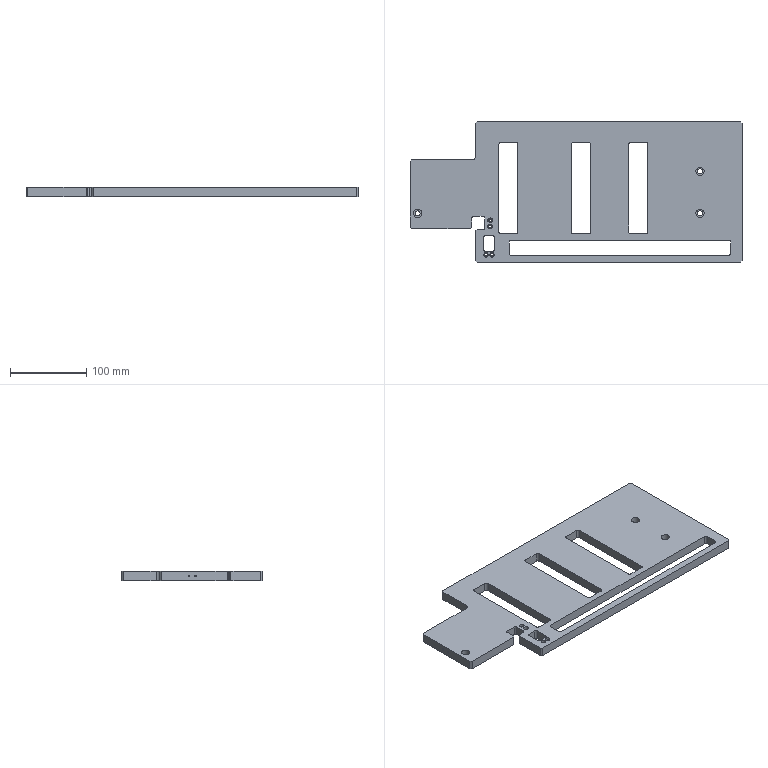NC program | NX | posted with a generic post | part box 435 x 184 x 12 mm
Lines 6316 to 7223 of 10210:
(HOLE_MILLING_COPY , TOOL : D4)
N12564 T11 M6
N12566 G54
N12568 G17 G0 G90 X-112.5 Y-37. S9500 M3
N12570 G43 Z30. H11
N12572 Z1.
N12574 G94 G3 X-112. Y-37.5 R0.5 F1500.
N12576 X-111.5 Y-37. R0.5
N12578 X-111.5 Y-37. Z0.5 I-1. J0.
N12580 X-111.5 Y-37. Z0. I-1. J0.
N12582 X-111.5 Y-37. Z-0.5 I-1. J0.
N12584 X-111.5 Y-37. Z-1. I-1. J0.
N12586 X-111.5 Y-37. Z-1.5 I-1. J0.
N12588 X-111.5 Y-37. Z-2. I-1. J0.
N12590 X-111.5 Y-37. Z-2.5 I-1. J0.
N12592 X-111.5 Y-37. Z-3. I-1. J0.
N12594 X-111.5 Y-37. Z-3.5 I-1. J0.
N12596 X-112.5 Y-36. R1.
N12598 X-111.5 Y-37. R-1.
N12600 X-112. Y-36.5 R0.5
N12602 X-112.5 Y-37. R0.5
N12604 G0 Z30.
N12606 Y-45.
N12608 Z1.
N12610 G3 X-112. Y-45.5 R0.5
N12612 X-111.5 Y-45. R0.5
N12614 X-111.5 Y-45. Z0.5 I-1. J0.
N12616 X-111.5 Y-45. Z0. I-1. J0.
N12618 X-111.5 Y-45. Z-0.5 I-1. J0.
N12620 X-111.5 Y-45. Z-1. I-1. J0.
N12622 X-111.5 Y-45. Z-1.5 I-1. J0.
N12624 X-111.5 Y-45. Z-2. I-1. J0.
N12626 X-111.5 Y-45. Z-2.5 I-1. J0.
N12628 X-111.5 Y-45. Z-3. I-1. J0.
N12630 X-111.5 Y-45. Z-3.5 I-1. J0.
N12632 X-112.5 Y-44. R1.
N12634 X-111.5 Y-45. R-1.
N12636 X-112. Y-44.5 R0.5
N12638 X-112.5 Y-45. R0.5
N12640 G0 Z30.
N12642 X-110. Y-82.5
N12644 Z1.
N12646 G3 X-109.5 Y-83. R0.5
N12648 X-109. Y-82.5 R0.5
N12650 X-109. Y-82.5 Z0.5 I-1. J0.
N12652 X-109. Y-82.5 Z0. I-1. J0.
N12654 X-109. Y-82.5 Z-0.5 I-1. J0.
N12656 X-109. Y-82.5 Z-1. I-1. J0.
N12658 X-109. Y-82.5 Z-1.5 I-1. J0.
N12660 X-109. Y-82.5 Z-2. I-1. J0.
N12662 X-109. Y-82.5 Z-2.5 I-1. J0.
N12664 X-109. Y-82.5 Z-3. I-1. J0.
N12666 X-109. Y-82.5 Z-3.5 I-1. J0.
N12668 X-110. Y-81.5 R1.
N12670 X-109. Y-82.5 R-1.
N12672 X-109.5 Y-82. R0.5
N12674 X-110. Y-82.5 R0.5
N12676 G0 Z30.
N12678 X-118.
N12680 Z1.
N12682 G3 X-117.5 Y-83. R0.5
N12684 X-117. Y-82.5 R0.5
N12686 X-117. Y-82.5 Z0.5 I-1. J0.
N12688 X-117. Y-82.5 Z0. I-1. J0.
N12690 X-117. Y-82.5 Z-0.5 I-1. J0.
N12692 X-117. Y-82.5 Z-1. I-1. J0.
N12694 X-117. Y-82.5 Z-1.5 I-1. J0.
N12696 X-117. Y-82.5 Z-2. I-1. J0.
N12698 X-117. Y-82.5 Z-2.5 I-1. J0.
N12700 X-117. Y-82.5 Z-3. I-1. J0.
N12702 X-117. Y-82.5 Z-3.5 I-1. J0.
N12704 X-118. Y-81.5 R1.
N12706 X-117. Y-82.5 R-1.
N12708 X-117.5 Y-82. R0.5
N12710 X-118. Y-82.5 R0.5
N12712 G0 Z30.
(ZLEVEL_PROFILE_COPY_1_COPY_COPY_1_COPY_COPY_COPY_1_COPY , TOOL : D4)
N12714 X71.8 Y-51.159
N12716 Z-0.5
N12718 G1 X71.2 Y-51.505 F1000.
N12720 G3 X71. Y-51.852 R0.4
N12722 G1 Y-52.5 F1500.
N12724 G3 X71.5 Y-53. R0.5
N12726 G1 X72.148
N12728 G3 X72.495 Y-52.8 R0.4
N12730 G1 X72.841 Y-52.2
N12732 G0 X71.8 Y-51.159 Z-1.
N12734 G1 X71.2 Y-51.505 F1000.
N12736 G3 X71. Y-51.852 R0.4
N12738 G1 Y-52.5 F1500.
N12740 G3 X71.5 Y-53. R0.5
N12742 G1 X72.148
N12744 G3 X72.495 Y-52.8 R0.4
N12746 G1 X72.841 Y-52.2
N12748 G0 X71.8 Y-51.159 Z-1.5
N12750 G1 X71.2 Y-51.505 F1000.
N12752 G3 X71. Y-51.852 R0.4
N12754 G1 Y-52.5 F1500.
N12756 G3 X71.5 Y-53. R0.5
N12758 G1 X72.148
N12760 G3 X72.495 Y-52.8 R0.4
N12762 G1 X72.841 Y-52.2
N12764 G0 X71.8 Y-51.159 Z-2.
N12766 G1 X71.2 Y-51.505 F1000.
N12768 G3 X71. Y-51.852 R0.4
N12770 G1 Y-52.5 F1500.
N12772 G3 X71.5 Y-53. R0.5
N12774 G1 X72.148
N12776 G3 X72.495 Y-52.8 R0.4
N12778 G1 X72.841 Y-52.2
N12780 G0 X71.8 Y-51.159 Z-2.5
N12782 G1 X71.2 Y-51.505 F1000.
N12784 G3 X71. Y-51.852 R0.4
N12786 G1 Y-52.5 F1500.
N12788 G3 X71.5 Y-53. R0.5
N12790 G1 X72.148
N12792 G3 X72.495 Y-52.8 R0.4
N12794 G1 X72.841 Y-52.2
N12796 G0 X71.8 Y-51.159 Z-3.
N12798 G1 X71.2 Y-51.505 F1000.
N12800 G3 X71. Y-51.852 R0.4
N12802 G1 Y-52.5 F1500.
N12804 G3 X71.5 Y-53. R0.5
N12806 G1 X72.148
N12808 G3 X72.495 Y-52.8 R0.4
N12810 G1 X72.841 Y-52.2
N12812 G0 X71.8 Y-51.159 Z-3.5
N12814 G1 X71.2 Y-51.505 F1000.
N12816 G3 X71. Y-51.852 R0.4
N12818 G1 Y-52.5 F1500.
N12820 G3 X71.5 Y-53. R0.5
N12822 G1 X72.148
N12824 G3 X72.495 Y-52.8 R0.4
N12826 G1 X72.841 Y-52.2
N12828 G0 X71.8 Y-51.159 Z-4.
N12830 G1 X71.2 Y-51.505 F1000.
N12832 G3 X71. Y-51.852 R0.4
N12834 G1 Y-52.5 F1500.
N12836 G3 X71.5 Y-53. R0.5
N12838 G1 X72.148
N12840 G3 X72.495 Y-52.8 R0.4
N12842 G1 X72.841 Y-52.2
N12844 G0 X71.8 Y-51.159 Z-4.5
N12846 G1 X71.2 Y-51.505 F1000.
N12848 G3 X71. Y-51.852 R0.4
N12850 G1 Y-52.5 F1500.
N12852 G3 X71.5 Y-53. R0.5
N12854 G1 X72.148
N12856 G3 X72.495 Y-52.8 R0.4
N12858 G1 X72.841 Y-52.2
N12860 G0 X71.8 Y-51.159 Z-5.
N12862 G1 X71.2 Y-51.505 F1000.
N12864 G3 X71. Y-51.852 R0.4
N12866 G1 Y-52.5 F1500.
N12868 G3 X71.5 Y-53. R0.5
N12870 G1 X72.148
N12872 G3 X72.495 Y-52.8 R0.4
N12874 G1 X72.841 Y-52.2
N12876 G0 X71.8 Y-51.159 Z-5.5
N12878 G1 X71.2 Y-51.505 F1000.
N12880 G3 X71. Y-51.852 R0.4
N12882 G1 Y-52.5 F1500.
N12884 G3 X71.5 Y-53. R0.5
N12886 G1 X72.148
N12888 G3 X72.495 Y-52.8 R0.4
N12890 G1 X72.841 Y-52.2
N12892 G0 X71.8 Y-51.159 Z-6.
N12894 G1 X71.2 Y-51.505 F1000.
N12896 G3 X71. Y-51.852 R0.4
N12898 G1 Y-52.5 F1500.
N12900 G3 X71.5 Y-53. R0.5
N12902 G1 X72.148
N12904 G3 X72.495 Y-52.8 R0.4
N12906 G1 X72.841 Y-52.2
N12908 G0 X71.8 Y-51.159 Z-6.5
N12910 G1 X71.2 Y-51.505 F1000.
N12912 G3 X71. Y-51.852 R0.4
N12914 G1 Y-52.5 F1500.
N12916 G3 X71.5 Y-53. R0.5
N12918 G1 X72.148
N12920 G3 X72.495 Y-52.8 R0.4
N12922 G1 X72.841 Y-52.2
N12924 G0 X71.8 Y-51.159 Z-7.
N12926 G1 X71.2 Y-51.505 F1000.
N12928 G3 X71. Y-51.852 R0.4
N12930 G1 Y-52.5 F1500.
N12932 G3 X71.5 Y-53. R0.5
N12934 G1 X72.148
N12936 G3 X72.495 Y-52.8 R0.4
N12938 G1 X72.841 Y-52.2
N12940 G0 X71.8 Y-51.159 Z-7.5
N12942 G1 X71.2 Y-51.505 F1000.
N12944 G3 X71. Y-51.852 R0.4
N12946 G1 Y-52.5 F1500.
N12948 G3 X71.5 Y-53. R0.5
N12950 G1 X72.148
N12952 G3 X72.495 Y-52.8 R0.4
N12954 G1 X72.841 Y-52.2
N12956 G0 X71.8 Y-51.159 Z-8.
N12958 G1 X71.2 Y-51.505 F1000.
N12960 G3 X71. Y-51.852 R0.4
N12962 G1 Y-52.5 F1500.
N12964 G3 X71.5 Y-53. R0.5
N12966 G1 X72.148
N12968 G3 X72.495 Y-52.8 R0.4
N12970 G1 X72.841 Y-52.2
N12972 G0 X71.8 Y-51.159 Z-8.5
N12974 G1 X71.2 Y-51.505 F1000.
N12976 G3 X71. Y-51.852 R0.4
N12978 G1 Y-52.5 F1500.
N12980 G3 X71.5 Y-53. R0.5
N12982 G1 X72.148
N12984 G3 X72.495 Y-52.8 R0.4
N12986 G1 X72.841 Y-52.2
N12988 G0 X71.8 Y-51.159 Z-9.
N12990 G1 X71.2 Y-51.505 F1000.
N12992 G3 X71. Y-51.852 R0.4
N12994 G1 Y-52.5 F1500.
N12996 G3 X71.5 Y-53. R0.5
N12998 G1 X72.148
N13000 G3 X72.495 Y-52.8 R0.4
N13002 G1 X72.841 Y-52.2
N13004 G0 X71.8 Y-51.159 Z-9.5
N13006 G1 X71.2 Y-51.505 F1000.
N13008 G3 X71. Y-51.852 R0.4
N13010 G1 Y-52.5 F1500.
N13012 G3 X71.5 Y-53. R0.5
N13014 G1 X72.148
N13016 G3 X72.495 Y-52.8 R0.4
N13018 G1 X72.841 Y-52.2
N13020 G0 X71.8 Y-51.159 Z-10.
N13022 G1 X71.2 Y-51.505 F1000.
N13024 G3 X71. Y-51.852 R0.4
N13026 G1 Y-52.5 F1500.
N13028 G3 X71.5 Y-53. R0.5
N13030 G1 X72.148
N13032 G3 X72.495 Y-52.8 R0.4
N13034 G1 X72.841 Y-52.2
N13036 G0 X71.8 Y-51.159 Z-10.5
N13038 G1 X71.2 Y-51.505 F1000.
N13040 G3 X71. Y-51.852 R0.4
N13042 G1 Y-52.5 F1500.
N13044 G3 X71.5 Y-53. R0.5
N13046 G1 X72.148
N13048 G3 X72.495 Y-52.8 R0.4
N13050 G1 X72.841 Y-52.2
N13052 G0 X71.8 Y-51.159 Z-11.
N13054 G1 X71.2 Y-51.505 F1000.
N13056 G3 X71. Y-51.852 R0.4
N13058 G1 Y-52.5 F1500.
N13060 G3 X71.5 Y-53. R0.5
N13062 G1 X72.148
N13064 G3 X72.495 Y-52.8 R0.4
N13066 G1 X72.841 Y-52.2
N13068 G0 X71.8 Y-51.159 Z-11.5
N13070 G1 X71.2 Y-51.505 F1000.
N13072 G3 X71. Y-51.852 R0.4
N13074 G1 Y-52.5 F1500.
N13076 G3 X71.5 Y-53. R0.5
N13078 G1 X72.148
N13080 G3 X72.495 Y-52.8 R0.4
N13082 G1 X72.841 Y-52.2
N13084 G0 X71.8 Y-51.159 Z-12.
N13086 G1 X71.2 Y-51.505 F1000.
N13088 G3 X71. Y-51.852 R0.4
N13090 G1 Y-52.5 F1500.
N13092 G3 X71.5 Y-53. R0.5
N13094 G1 X72.148
N13096 G3 X72.495 Y-52.8 R0.4
N13098 G1 X72.841 Y-52.2
N13100 G0 Z30.
N13102 X90.159
N13104 Z-0.5
N13106 G1 X90.505 Y-52.8 F1000.
N13108 G3 X90.852 Y-53. R0.4
N13110 G1 X91.5 F1500.
N13112 G3 X92. Y-52.5 R0.5
N13114 G1 Y-51.852
N13116 G3 X91.8 Y-51.506 R0.4
N13118 G1 X91.2 Y-51.159
N13120 G0 X90.159 Y-52.2 Z-1.
N13122 G1 X90.505 Y-52.8 F1000.
N13124 G3 X90.852 Y-53. R0.4
N13126 G1 X91.5 F1500.
N13128 G3 X92. Y-52.5 R0.5
N13130 G1 Y-51.852
N13132 G3 X91.8 Y-51.506 R0.4
N13134 G1 X91.2 Y-51.159
N13136 G0 X90.159 Y-52.2 Z-1.5
N13138 G1 X90.505 Y-52.8 F1000.
N13140 G3 X90.852 Y-53. R0.4
N13142 G1 X91.5 F1500.
N13144 G3 X92. Y-52.5 R0.5
N13146 G1 Y-51.852
N13148 G3 X91.8 Y-51.506 R0.4
N13150 G1 X91.2 Y-51.159
N13152 G0 X90.159 Y-52.2 Z-2.
N13154 G1 X90.505 Y-52.8 F1000.
N13156 G3 X90.852 Y-53. R0.4
N13158 G1 X91.5 F1500.
N13160 G3 X92. Y-52.5 R0.5
N13162 G1 Y-51.852
N13164 G3 X91.8 Y-51.506 R0.4
N13166 G1 X91.2 Y-51.159
N13168 G0 X90.159 Y-52.2 Z-2.5
N13170 G1 X90.505 Y-52.8 F1000.
N13172 G3 X90.852 Y-53. R0.4
N13174 G1 X91.5 F1500.
N13176 G3 X92. Y-52.5 R0.5
N13178 G1 Y-51.852
N13180 G3 X91.8 Y-51.506 R0.4
N13182 G1 X91.2 Y-51.159
N13184 G0 X90.159 Y-52.2 Z-3.
N13186 G1 X90.505 Y-52.8 F1000.
N13188 G3 X90.852 Y-53. R0.4
N13190 G1 X91.5 F1500.
N13192 G3 X92. Y-52.5 R0.5
N13194 G1 Y-51.852
N13196 G3 X91.8 Y-51.506 R0.4
N13198 G1 X91.2 Y-51.159
N13200 G0 X90.159 Y-52.2 Z-3.5
N13202 G1 X90.505 Y-52.8 F1000.
N13204 G3 X90.852 Y-53. R0.4
N13206 G1 X91.5 F1500.
N13208 G3 X92. Y-52.5 R0.5
N13210 G1 Y-51.852
N13212 G3 X91.8 Y-51.506 R0.4
N13214 G1 X91.2 Y-51.159
N13216 G0 X90.159 Y-52.2 Z-4.
N13218 G1 X90.505 Y-52.8 F1000.
N13220 G3 X90.852 Y-53. R0.4
N13222 G1 X91.5 F1500.
N13224 G3 X92. Y-52.5 R0.5
N13226 G1 Y-51.852
N13228 G3 X91.8 Y-51.506 R0.4
N13230 G1 X91.2 Y-51.159
N13232 G0 X90.159 Y-52.2 Z-4.5
N13234 G1 X90.505 Y-52.8 F1000.
N13236 G3 X90.852 Y-53. R0.4
N13238 G1 X91.5 F1500.
N13240 G3 X92. Y-52.5 R0.5
N13242 G1 Y-51.852
N13244 G3 X91.8 Y-51.506 R0.4
N13246 G1 X91.2 Y-51.159
N13248 G0 X90.159 Y-52.2 Z-5.
N13250 G1 X90.505 Y-52.8 F1000.
N13252 G3 X90.852 Y-53. R0.4
N13254 G1 X91.5 F1500.
N13256 G3 X92. Y-52.5 R0.5
N13258 G1 Y-51.852
N13260 G3 X91.8 Y-51.506 R0.4
N13262 G1 X91.2 Y-51.159
N13264 G0 X90.159 Y-52.2 Z-5.5
N13266 G1 X90.505 Y-52.8 F1000.
N13268 G3 X90.852 Y-53. R0.4
N13270 G1 X91.5 F1500.
N13272 G3 X92. Y-52.5 R0.5
N13274 G1 Y-51.852
N13276 G3 X91.8 Y-51.506 R0.4
N13278 G1 X91.2 Y-51.159
N13280 G0 X90.159 Y-52.2 Z-6.
N13282 G1 X90.505 Y-52.8 F1000.
N13284 G3 X90.852 Y-53. R0.4
N13286 G1 X91.5 F1500.
N13288 G3 X92. Y-52.5 R0.5
N13290 G1 Y-51.852
N13292 G3 X91.8 Y-51.506 R0.4
N13294 G1 X91.2 Y-51.159
N13296 G0 X90.159 Y-52.2 Z-6.5
N13298 G1 X90.505 Y-52.8 F1000.
N13300 G3 X90.852 Y-53. R0.4
N13302 G1 X91.5 F1500.
N13304 G3 X92. Y-52.5 R0.5
N13306 G1 Y-51.852
N13308 G3 X91.8 Y-51.506 R0.4
N13310 G1 X91.2 Y-51.159
N13312 G0 X90.159 Y-52.2 Z-7.
N13314 G1 X90.505 Y-52.8 F1000.
N13316 G3 X90.852 Y-53. R0.4
N13318 G1 X91.5 F1500.
N13320 G3 X92. Y-52.5 R0.5
N13322 G1 Y-51.852
N13324 G3 X91.8 Y-51.506 R0.4
N13326 G1 X91.2 Y-51.159
N13328 G0 X90.159 Y-52.2 Z-7.5
N13330 G1 X90.505 Y-52.8 F1000.
N13332 G3 X90.852 Y-53. R0.4
N13334 G1 X91.5 F1500.
N13336 G3 X92. Y-52.5 R0.5
N13338 G1 Y-51.852
N13340 G3 X91.8 Y-51.506 R0.4
N13342 G1 X91.2 Y-51.159
N13344 G0 X90.159 Y-52.2 Z-8.
N13346 G1 X90.505 Y-52.8 F1000.
N13348 G3 X90.852 Y-53. R0.4
N13350 G1 X91.5 F1500.
N13352 G3 X92. Y-52.5 R0.5
N13354 G1 Y-51.852
N13356 G3 X91.8 Y-51.506 R0.4
N13358 G1 X91.2 Y-51.159
N13360 G0 X90.159 Y-52.2 Z-8.5
N13362 G1 X90.505 Y-52.8 F1000.
N13364 G3 X90.852 Y-53. R0.4
N13366 G1 X91.5 F1500.
N13368 G3 X92. Y-52.5 R0.5
N13370 G1 Y-51.852
N13372 G3 X91.8 Y-51.506 R0.4
N13374 G1 X91.2 Y-51.159
N13376 G0 X90.159 Y-52.2 Z-9.
N13378 G1 X90.505 Y-52.8 F1000.
N13380 G3 X90.852 Y-53. R0.4
N13382 G1 X91.5 F1500.
N13384 G3 X92. Y-52.5 R0.5
N13386 G1 Y-51.852
N13388 G3 X91.8 Y-51.506 R0.4
N13390 G1 X91.2 Y-51.159
N13392 G0 X90.159 Y-52.2 Z-9.5
N13394 G1 X90.505 Y-52.8 F1000.
N13396 G3 X90.852 Y-53. R0.4
N13398 G1 X91.5 F1500.
N13400 G3 X92. Y-52.5 R0.5
N13402 G1 Y-51.852
N13404 G3 X91.8 Y-51.506 R0.4
N13406 G1 X91.2 Y-51.159
N13408 G0 X90.159 Y-52.2 Z-10.
N13410 G1 X90.505 Y-52.8 F1000.
N13412 G3 X90.852 Y-53. R0.4
N13414 G1 X91.5 F1500.
N13416 G3 X92. Y-52.5 R0.5
N13418 G1 Y-51.852
N13420 G3 X91.8 Y-51.506 R0.4
N13422 G1 X91.2 Y-51.159
N13424 G0 X90.159 Y-52.2 Z-10.5
N13426 G1 X90.505 Y-52.8 F1000.
N13428 G3 X90.852 Y-53. R0.4
N13430 G1 X91.5 F1500.
N13432 G3 X92. Y-52.5 R0.5
N13434 G1 Y-51.852
N13436 G3 X91.8 Y-51.506 R0.4
N13438 G1 X91.2 Y-51.159
N13440 G0 X90.159 Y-52.2 Z-11.
N13442 G1 X90.505 Y-52.8 F1000.
N13444 G3 X90.852 Y-53. R0.4
N13446 G1 X91.5 F1500.
N13448 G3 X92. Y-52.5 R0.5
N13450 G1 Y-51.852
N13452 G3 X91.8 Y-51.506 R0.4
N13454 G1 X91.2 Y-51.159
N13456 G0 X90.159 Y-52.2 Z-11.5
N13458 G1 X90.505 Y-52.8 F1000.
N13460 G3 X90.852 Y-53. R0.4
N13462 G1 X91.5 F1500.
N13464 G3 X92. Y-52.5 R0.5
N13466 G1 Y-51.852
N13468 G3 X91.8 Y-51.506 R0.4
N13470 G1 X91.2 Y-51.159
N13472 G0 X90.159 Y-52.2 Z-12.
N13474 G1 X90.505 Y-52.8 F1000.
N13476 G3 X90.852 Y-53. R0.4
N13478 G1 X91.5 F1500.
N13480 G3 X92. Y-52.5 R0.5
N13482 G1 Y-51.852
N13484 G3 X91.8 Y-51.506 R0.4
N13486 G1 X91.2 Y-51.159
N13488 G0 Z30.
N13490 Y61.159
N13492 Z-0.5
N13494 G1 X91.8 Y61.506 F1000.
N13496 G3 X92. Y61.852 R0.4
N13498 G1 Y62.5 F1500.
N13500 G3 X91.5 Y63. R0.5
N13502 G1 X90.852
N13504 G3 X90.505 Y62.8 R0.4
N13506 G1 X90.159 Y62.2
N13508 G0 X91.2 Y61.159 Z-1.
N13510 G1 X91.8 Y61.506 F1000.
N13512 G3 X92. Y61.852 R0.4
N13514 G1 Y62.5 F1500.
N13516 G3 X91.5 Y63. R0.5
N13518 G1 X90.852
N13520 G3 X90.505 Y62.8 R0.4
N13522 G1 X90.159 Y62.2
N13524 G0 X91.2 Y61.159 Z-1.5
N13526 G1 X91.8 Y61.506 F1000.
N13528 G3 X92. Y61.852 R0.4
N13530 G1 Y62.5 F1500.
N13532 G3 X91.5 Y63. R0.5
N13534 G1 X90.852
N13536 G3 X90.505 Y62.8 R0.4
N13538 G1 X90.159 Y62.2
N13540 G0 X91.2 Y61.159 Z-2.
N13542 G1 X91.8 Y61.506 F1000.
N13544 G3 X92. Y61.852 R0.4
N13546 G1 Y62.5 F1500.
N13548 G3 X91.5 Y63. R0.5
N13550 G1 X90.852
N13552 G3 X90.505 Y62.8 R0.4
N13554 G1 X90.159 Y62.2
N13556 G0 X91.2 Y61.159 Z-2.5
N13558 G1 X91.8 Y61.506 F1000.
N13560 G3 X92. Y61.852 R0.4
N13562 G1 Y62.5 F1500.
N13564 G3 X91.5 Y63. R0.5
N13566 G1 X90.852
N13568 G3 X90.505 Y62.8 R0.4
N13570 G1 X90.159 Y62.2
N13572 G0 X91.2 Y61.159 Z-3.
N13574 G1 X91.8 Y61.506 F1000.
N13576 G3 X92. Y61.852 R0.4
N13578 G1 Y62.5 F1500.
N13580 G3 X91.5 Y63. R0.5
N13582 G1 X90.852
N13584 G3 X90.505 Y62.8 R0.4
N13586 G1 X90.159 Y62.2
N13588 G0 X91.2 Y61.159 Z-3.5
N13590 G1 X91.8 Y61.506 F1000.
N13592 G3 X92. Y61.852 R0.4
N13594 G1 Y62.5 F1500.
N13596 G3 X91.5 Y63. R0.5
N13598 G1 X90.852
N13600 G3 X90.505 Y62.8 R0.4
N13602 G1 X90.159 Y62.2
N13604 G0 X91.2 Y61.159 Z-4.
N13606 G1 X91.8 Y61.506 F1000.
N13608 G3 X92. Y61.852 R0.4
N13610 G1 Y62.5 F1500.
N13612 G3 X91.5 Y63. R0.5
N13614 G1 X90.852
N13616 G3 X90.505 Y62.8 R0.4
N13618 G1 X90.159 Y62.2
N13620 G0 X91.2 Y61.159 Z-4.5
N13622 G1 X91.8 Y61.506 F1000.
N13624 G3 X92. Y61.852 R0.4
N13626 G1 Y62.5 F1500.
N13628 G3 X91.5 Y63. R0.5
N13630 G1 X90.852
N13632 G3 X90.505 Y62.8 R0.4
N13634 G1 X90.159 Y62.2
N13636 G0 X91.2 Y61.159 Z-5.
N13638 G1 X91.8 Y61.506 F1000.
N13640 G3 X92. Y61.852 R0.4
N13642 G1 Y62.5 F1500.
N13644 G3 X91.5 Y63. R0.5
N13646 G1 X90.852
N13648 G3 X90.505 Y62.8 R0.4
N13650 G1 X90.159 Y62.2
N13652 G0 X91.2 Y61.159 Z-5.5
N13654 G1 X91.8 Y61.506 F1000.
N13656 G3 X92. Y61.852 R0.4
N13658 G1 Y62.5 F1500.
N13660 G3 X91.5 Y63. R0.5
N13662 G1 X90.852
N13664 G3 X90.505 Y62.8 R0.4
N13666 G1 X90.159 Y62.2
N13668 G0 X91.2 Y61.159 Z-6.
N13670 G1 X91.8 Y61.506 F1000.
N13672 G3 X92. Y61.852 R0.4
N13674 G1 Y62.5 F1500.
N13676 G3 X91.5 Y63. R0.5
N13678 G1 X90.852
N13680 G3 X90.505 Y62.8 R0.4
N13682 G1 X90.159 Y62.2
N13684 G0 X91.2 Y61.159 Z-6.5
N13686 G1 X91.8 Y61.506 F1000.
N13688 G3 X92. Y61.852 R0.4
N13690 G1 Y62.5 F1500.
N13692 G3 X91.5 Y63. R0.5
N13694 G1 X90.852
N13696 G3 X90.505 Y62.8 R0.4
N13698 G1 X90.159 Y62.2
N13700 G0 X91.2 Y61.159 Z-7.
N13702 G1 X91.8 Y61.506 F1000.
N13704 G3 X92. Y61.852 R0.4
N13706 G1 Y62.5 F1500.
N13708 G3 X91.5 Y63. R0.5
N13710 G1 X90.852
N13712 G3 X90.505 Y62.8 R0.4
N13714 G1 X90.159 Y62.2
N13716 G0 X91.2 Y61.159 Z-7.5
N13718 G1 X91.8 Y61.506 F1000.
N13720 G3 X92. Y61.852 R0.4
N13722 G1 Y62.5 F1500.
N13724 G3 X91.5 Y63. R0.5
N13726 G1 X90.852
N13728 G3 X90.505 Y62.8 R0.4
N13730 G1 X90.159 Y62.2
N13732 G0 X91.2 Y61.159 Z-8.
N13734 G1 X91.8 Y61.506 F1000.
N13736 G3 X92. Y61.852 R0.4
N13738 G1 Y62.5 F1500.
N13740 G3 X91.5 Y63. R0.5
N13742 G1 X90.852
N13744 G3 X90.505 Y62.8 R0.4
N13746 G1 X90.159 Y62.2
N13748 G0 X91.2 Y61.159 Z-8.5
N13750 G1 X91.8 Y61.506 F1000.
N13752 G3 X92. Y61.852 R0.4
N13754 G1 Y62.5 F1500.
N13756 G3 X91.5 Y63. R0.5
N13758 G1 X90.852
N13760 G3 X90.505 Y62.8 R0.4
N13762 G1 X90.159 Y62.2
N13764 G0 X91.2 Y61.159 Z-9.
N13766 G1 X91.8 Y61.506 F1000.
N13768 G3 X92. Y61.852 R0.4
N13770 G1 Y62.5 F1500.
N13772 G3 X91.5 Y63. R0.5
N13774 G1 X90.852
N13776 G3 X90.505 Y62.8 R0.4
N13778 G1 X90.159 Y62.2
N13780 G0 X91.2 Y61.159 Z-9.5
N13782 G1 X91.8 Y61.506 F1000.
N13784 G3 X92. Y61.852 R0.4
N13786 G1 Y62.5 F1500.
N13788 G3 X91.5 Y63. R0.5
N13790 G1 X90.852
N13792 G3 X90.505 Y62.8 R0.4
N13794 G1 X90.159 Y62.2
N13796 G0 X91.2 Y61.159 Z-10.
N13798 G1 X91.8 Y61.506 F1000.
N13800 G3 X92. Y61.852 R0.4
N13802 G1 Y62.5 F1500.
N13804 G3 X91.5 Y63. R0.5
N13806 G1 X90.852
N13808 G3 X90.505 Y62.8 R0.4
N13810 G1 X90.159 Y62.2
N13812 G0 X91.2 Y61.159 Z-10.5
N13814 G1 X91.8 Y61.506 F1000.
N13816 G3 X92. Y61.852 R0.4
N13818 G1 Y62.5 F1500.
N13820 G3 X91.5 Y63. R0.5
N13822 G1 X90.852
N13824 G3 X90.505 Y62.8 R0.4
N13826 G1 X90.159 Y62.2
N13828 G0 X91.2 Y61.159 Z-11.
N13830 G1 X91.8 Y61.506 F1000.
N13832 G3 X92. Y61.852 R0.4
N13834 G1 Y62.5 F1500.
N13836 G3 X91.5 Y63. R0.5
N13838 G1 X90.852
N13840 G3 X90.505 Y62.8 R0.4
N13842 G1 X90.159 Y62.2
N13844 G0 X91.2 Y61.159 Z-11.5
N13846 G1 X91.8 Y61.506 F1000.
N13848 G3 X92. Y61.852 R0.4
N13850 G1 Y62.5 F1500.
N13852 G3 X91.5 Y63. R0.5
N13854 G1 X90.852
N13856 G3 X90.505 Y62.8 R0.4
N13858 G1 X90.159 Y62.2
N13860 G0 X91.2 Y61.159 Z-12.
N13862 G1 X91.8 Y61.506 F1000.
N13864 G3 X92. Y61.852 R0.4
N13866 G1 Y62.5 F1500.
N13868 G3 X91.5 Y63. R0.5
N13870 G1 X90.852
N13872 G3 X90.505 Y62.8 R0.4
N13874 G1 X90.159 Y62.2
N13876 G0 Z30.
N13878 X72.84
N13880 Z-0.5
N13882 G1 X72.494 Y62.8 F1000.
N13884 G3 X72.147 Y63. R0.4
N13886 G1 X71.5 F1500.
N13888 G3 X71. Y62.5 R0.5
N13890 G1 Y61.853
N13892 G3 X71.2 Y61.506 R0.4
N13894 G1 X71.8 Y61.16
N13896 G0 X72.84 Y62.2 Z-1.
N13898 G1 X72.494 Y62.8 F1000.
N13900 G3 X72.147 Y63. R0.4
N13902 G1 X71.5 F1500.
N13904 G3 X71. Y62.5 R0.5
N13906 G1 Y61.853
N13908 G3 X71.2 Y61.506 R0.4
N13910 G1 X71.8 Y61.16
N13912 G0 X72.84 Y62.2 Z-1.5
N13914 G1 X72.494 Y62.8 F1000.
N13916 G3 X72.147 Y63. R0.4
N13918 G1 X71.5 F1500.
N13920 G3 X71. Y62.5 R0.5
N13922 G1 Y61.853
N13924 G3 X71.2 Y61.506 R0.4
N13926 G1 X71.8 Y61.16
N13928 G0 X72.84 Y62.2 Z-2.
N13930 G1 X72.494 Y62.8 F1000.
N13932 G3 X72.147 Y63. R0.4
N13934 G1 X71.5 F1500.
N13936 G3 X71. Y62.5 R0.5
N13938 G1 Y61.853
N13940 G3 X71.2 Y61.506 R0.4
N13942 G1 X71.8 Y61.16
N13944 G0 X72.84 Y62.2 Z-2.5
N13946 G1 X72.494 Y62.8 F1000.
N13948 G3 X72.147 Y63. R0.4
N13950 G1 X71.5 F1500.
N13952 G3 X71. Y62.5 R0.5
N13954 G1 Y61.853
N13956 G3 X71.2 Y61.506 R0.4
N13958 G1 X71.8 Y61.16
N13960 G0 X72.84 Y62.2 Z-3.
N13962 G1 X72.494 Y62.8 F1000.
N13964 G3 X72.147 Y63. R0.4
N13966 G1 X71.5 F1500.
N13968 G3 X71. Y62.5 R0.5
N13970 G1 Y61.853
N13972 G3 X71.2 Y61.506 R0.4
N13974 G1 X71.8 Y61.16
N13976 G0 X72.84 Y62.2 Z-3.5
N13978 G1 X72.494 Y62.8 F1000.
N13980 G3 X72.147 Y63. R0.4
N13982 G1 X71.5 F1500.
N13984 G3 X71. Y62.5 R0.5
N13986 G1 Y61.853
N13988 G3 X71.2 Y61.506 R0.4
N13990 G1 X71.8 Y61.16
N13992 G0 X72.84 Y62.2 Z-4.
N13994 G1 X72.494 Y62.8 F1000.
N13996 G3 X72.147 Y63. R0.4
N13998 G1 X71.5 F1500.
N14000 G3 X71. Y62.5 R0.5
N14002 G1 Y61.853
N14004 G3 X71.2 Y61.506 R0.4
N14006 G1 X71.8 Y61.16
N14008 G0 X72.84 Y62.2 Z-4.5
N14010 G1 X72.494 Y62.8 F1000.
N14012 G3 X72.147 Y63. R0.4
N14014 G1 X71.5 F1500.
N14016 G3 X71. Y62.5 R0.5
N14018 G1 Y61.853
N14020 G3 X71.2 Y61.506 R0.4
N14022 G1 X71.8 Y61.16
N14024 G0 X72.84 Y62.2 Z-5.
N14026 G1 X72.494 Y62.8 F1000.
N14028 G3 X72.147 Y63. R0.4
N14030 G1 X71.5 F1500.
N14032 G3 X71. Y62.5 R0.5
N14034 G1 Y61.853
N14036 G3 X71.2 Y61.506 R0.4
N14038 G1 X71.8 Y61.16
N14040 G0 X72.84 Y62.2 Z-5.5
N14042 G1 X72.494 Y62.8 F1000.
N14044 G3 X72.147 Y63. R0.4
N14046 G1 X71.5 F1500.
N14048 G3 X71. Y62.5 R0.5
N14050 G1 Y61.853
N14052 G3 X71.2 Y61.506 R0.4
N14054 G1 X71.8 Y61.16
N14056 G0 X72.84 Y62.2 Z-6.
N14058 G1 X72.494 Y62.8 F1000.
N14060 G3 X72.147 Y63. R0.4
N14062 G1 X71.5 F1500.
N14064 G3 X71. Y62.5 R0.5
N14066 G1 Y61.853
N14068 G3 X71.2 Y61.506 R0.4
N14070 G1 X71.8 Y61.16
N14072 G0 X72.84 Y62.2 Z-6.5
N14074 G1 X72.494 Y62.8 F1000.
N14076 G3 X72.147 Y63. R0.4
N14078 G1 X71.5 F1500.
N14080 G3 X71. Y62.5 R0.5
N14082 G1 Y61.853
N14084 G3 X71.2 Y61.506 R0.4
N14086 G1 X71.8 Y61.16
N14088 G0 X72.84 Y62.2 Z-7.
N14090 G1 X72.494 Y62.8 F1000.
N14092 G3 X72.147 Y63. R0.4
N14094 G1 X71.5 F1500.
N14096 G3 X71. Y62.5 R0.5
N14098 G1 Y61.853
N14100 G3 X71.2 Y61.506 R0.4
N14102 G1 X71.8 Y61.16
N14104 G0 X72.84 Y62.2 Z-7.5
N14106 G1 X72.494 Y62.8 F1000.
N14108 G3 X72.147 Y63. R0.4
N14110 G1 X71.5 F1500.
N14112 G3 X71. Y62.5 R0.5
N14114 G1 Y61.853
N14116 G3 X71.2 Y61.506 R0.4
N14118 G1 X71.8 Y61.16
N14120 G0 X72.84 Y62.2 Z-8.
N14122 G1 X72.494 Y62.8 F1000.
N14124 G3 X72.147 Y63. R0.4
N14126 G1 X71.5 F1500.
N14128 G3 X71. Y62.5 R0.5
N14130 G1 Y61.853
N14132 G3 X71.2 Y61.506 R0.4
N14134 G1 X71.8 Y61.16
N14136 G0 X72.84 Y62.2 Z-8.5
N14138 G1 X72.494 Y62.8 F1000.
N14140 G3 X72.147 Y63. R0.4
N14142 G1 X71.5 F1500.
N14144 G3 X71. Y62.5 R0.5
N14146 G1 Y61.853
N14148 G3 X71.2 Y61.506 R0.4
N14150 G1 X71.8 Y61.16
N14152 G0 X72.84 Y62.2 Z-9.
N14154 G1 X72.494 Y62.8 F1000.
N14156 G3 X72.147 Y63. R0.4
N14158 G1 X71.5 F1500.
N14160 G3 X71. Y62.5 R0.5
N14162 G1 Y61.853
N14164 G3 X71.2 Y61.506 R0.4
N14166 G1 X71.8 Y61.16
N14168 G0 X72.84 Y62.2 Z-9.5
N14170 G1 X72.494 Y62.8 F1000.
N14172 G3 X72.147 Y63. R0.4
N14174 G1 X71.5 F1500.
N14176 G3 X71. Y62.5 R0.5
N14178 G1 Y61.853
N14180 G3 X71.2 Y61.506 R0.4
N14182 G1 X71.8 Y61.16
N14184 G0 X72.84 Y62.2 Z-10.
N14186 G1 X72.494 Y62.8 F1000.
N14188 G3 X72.147 Y63. R0.4
N14190 G1 X71.5 F1500.
N14192 G3 X71. Y62.5 R0.5
N14194 G1 Y61.853
N14196 G3 X71.2 Y61.506 R0.4
N14198 G1 X71.8 Y61.16
N14200 G0 X72.84 Y62.2 Z-10.5
N14202 G1 X72.494 Y62.8 F1000.
N14204 G3 X72.147 Y63. R0.4
N14206 G1 X71.5 F1500.
N14208 G3 X71. Y62.5 R0.5
N14210 G1 Y61.853
N14212 G3 X71.2 Y61.506 R0.4
N14214 G1 X71.8 Y61.16
N14216 G0 X72.84 Y62.2 Z-11.
N14218 G1 X72.494 Y62.8 F1000.
N14220 G3 X72.147 Y63. R0.4
N14222 G1 X71.5 F1500.
N14224 G3 X71. Y62.5 R0.5
N14226 G1 Y61.853
N14228 G3 X71.2 Y61.506 R0.4
N14230 G1 X71.8 Y61.16
N14232 G0 X72.84 Y62.2 Z-11.5
N14234 G1 X72.494 Y62.8 F1000.
N14236 G3 X72.147 Y63. R0.4
N14238 G1 X71.5 F1500.
N14240 G3 X71. Y62.5 R0.5
N14242 G1 Y61.853
N14244 G3 X71.2 Y61.506 R0.4
N14246 G1 X71.8 Y61.16
N14248 G0 X72.84 Y62.2 Z-12.
N14250 G1 X72.494 Y62.8 F1000.
N14252 G3 X72.147 Y63. R0.4
N14254 G1 X71.5 F1500.
N14256 G3 X71. Y62.5 R0.5
N14258 G1 Y61.853
N14260 G3 X71.2 Y61.506 R0.4
N14262 G1 X71.8 Y61.16
N14264 G0 Z53.
N14266 X-3.2 Y-51.147
N14268 Z-0.5
N14270 G1 X-3.8 Y-51.493 F1000.
N14272 G3 X-4. Y-51.84 R0.4
N14274 G1 Y-52.5 F1500.
N14276 G3 X-3.5 Y-53. R0.5
N14278 G1 X-2.847
N14280 G3 X-2.501 Y-52.8 R0.4
N14282 G1 X-2.155 Y-52.2
N14284 G0 X-3.2 Y-51.147 Z-1.
N14286 G1 X-3.8 Y-51.493 F1000.
N14288 G3 X-4. Y-51.84 R0.4
N14290 G1 Y-52.5 F1500.
N14292 G3 X-3.5 Y-53. R0.5
N14294 G1 X-2.847
N14296 G3 X-2.501 Y-52.8 R0.4
N14298 G1 X-2.155 Y-52.2
N14300 G0 X-3.2 Y-51.147 Z-1.5
N14302 G1 X-3.8 Y-51.493 F1000.
N14304 G3 X-4. Y-51.84 R0.4
N14306 G1 Y-52.5 F1500.
N14308 G3 X-3.5 Y-53. R0.5
N14310 G1 X-2.847
N14312 G3 X-2.501 Y-52.8 R0.4
N14314 G1 X-2.155 Y-52.2
N14316 G0 X-3.2 Y-51.147 Z-2.
N14318 G1 X-3.8 Y-51.493 F1000.
N14320 G3 X-4. Y-51.84 R0.4
N14322 G1 Y-52.5 F1500.
N14324 G3 X-3.5 Y-53. R0.5
N14326 G1 X-2.847
N14328 G3 X-2.501 Y-52.8 R0.4
N14330 G1 X-2.155 Y-52.2
N14332 G0 X-3.2 Y-51.147 Z-2.5
N14334 G1 X-3.8 Y-51.493 F1000.
N14336 G3 X-4. Y-51.84 R0.4
N14338 G1 Y-52.5 F1500.
N14340 G3 X-3.5 Y-53. R0.5
N14342 G1 X-2.847
N14344 G3 X-2.501 Y-52.8 R0.4
N14346 G1 X-2.155 Y-52.2
N14348 G0 X-3.2 Y-51.147 Z-3.
N14350 G1 X-3.8 Y-51.493 F1000.
N14352 G3 X-4. Y-51.84 R0.4
N14354 G1 Y-52.5 F1500.
N14356 G3 X-3.5 Y-53. R0.5
N14358 G1 X-2.847
N14360 G3 X-2.501 Y-52.8 R0.4
N14362 G1 X-2.155 Y-52.2
N14364 G0 X-3.2 Y-51.147 Z-3.5
N14366 G1 X-3.8 Y-51.493 F1000.